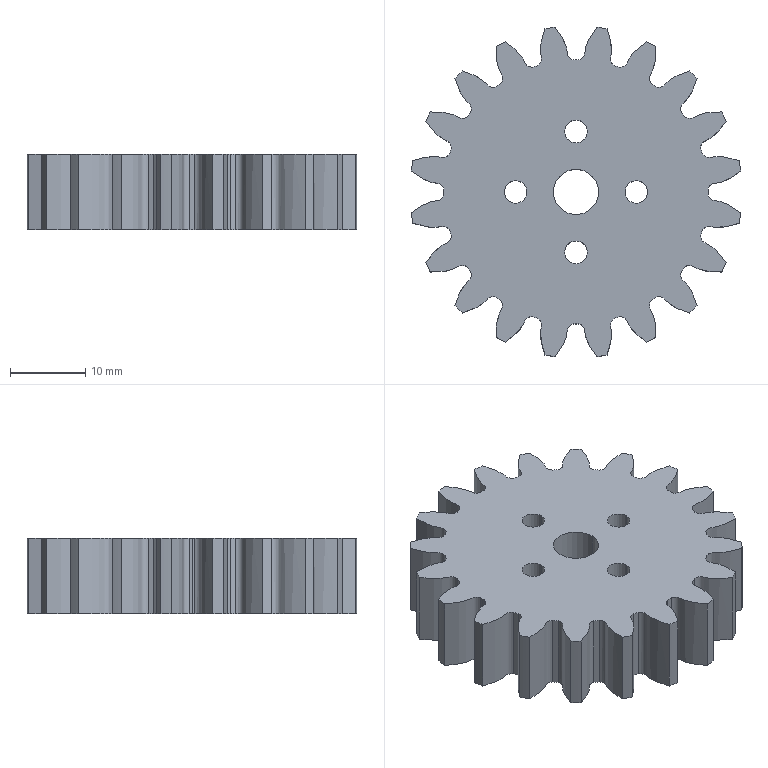Part | STEP file | Chuck drive gear | 1 solid | 96 faces | box 43.654 x 43.654 x 10 mm | volume 11238 mm3 | cylinder 53 | spline 40 | plane 3 | commonest cylinder face diameters 35 x21 44 x20 3 x8 6 x2 23 x2